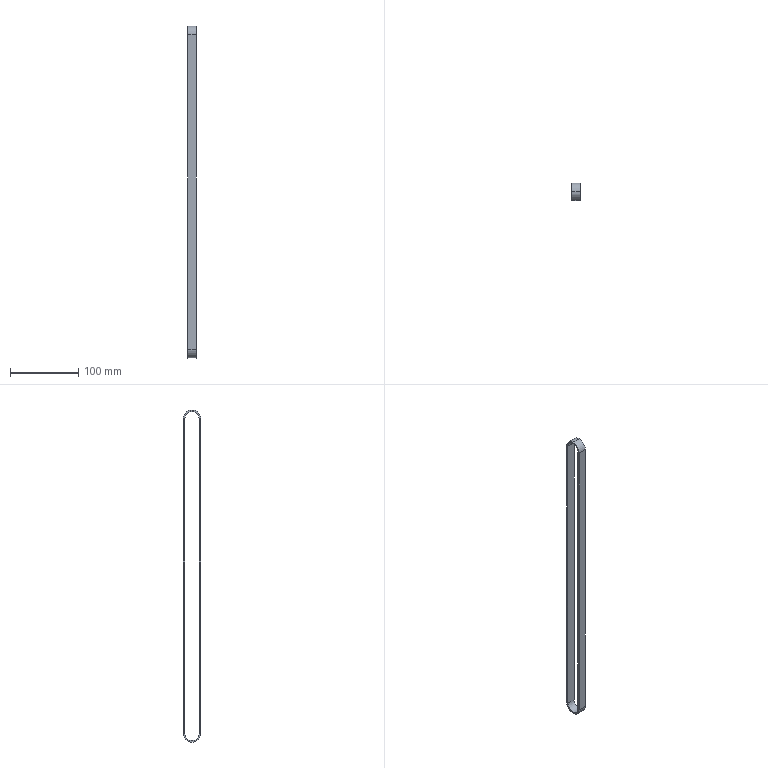Part | NX | features BREP 1 | 1 solid | 12 faces | box 12.7 x 25.408 x 484.908 mm | volume 28965 mm3 | plane 6 | cylinder 6 | commonest cylinder face diameters 20.808 x3 25.408 x3
STEP:
#1=CARTESIAN_POINT('',(-6.35,10.404,0.));
#2=VERTEX_POINT('',#1);
#3=CARTESIAN_POINT('',(6.35,10.404,0.));
#4=VERTEX_POINT('',#3);
#5=CARTESIAN_POINT('',(-6.35,10.404,0.));
#6=CARTESIAN_POINT('',(-2.117,10.404,0.));
#7=CARTESIAN_POINT('',(2.117,10.404,0.));
#8=CARTESIAN_POINT('',(6.35,10.404,0.));
#9=B_SPLINE_CURVE_WITH_KNOTS('',3,(#5,#6,#7,#8),.UNSPECIFIED.,.F.,.F.,(4,4),(0.,1.),.UNSPECIFIED.);
#10=EDGE_CURVE('',#2,#4,#9,.T.);
#11=ORIENTED_EDGE('',*,*,#10,.F.);
#12=CARTESIAN_POINT('',(-6.35,10.404,-459.5));
#13=VERTEX_POINT('',#12);
#14=CARTESIAN_POINT('',(-6.35,10.404,-459.5));
#15=DIRECTION('',(0.,0.,1.));
#16=VECTOR('',#15,1000.);
#17=LINE('',#14,#16);
#18=EDGE_CURVE('',#13,#2,#17,.T.);
#19=ORIENTED_EDGE('',*,*,#18,.F.);
#20=CARTESIAN_POINT('',(6.35,10.404,-459.5));
#21=VERTEX_POINT('',#20);
#22=CARTESIAN_POINT('',(6.35,10.404,-459.5));
#23=DIRECTION('',(1.,0.,0.));
#24=VECTOR('',#23,1000.);
#25=LINE('',#22,#24);
#26=EDGE_CURVE('',#13,#21,#25,.T.);
#27=ORIENTED_EDGE('',*,*,#26,.T.);
#28=CARTESIAN_POINT('',(6.35,10.404,-459.5));
#29=DIRECTION('',(0.,0.,1.));
#30=VECTOR('',#29,1000.);
#31=LINE('',#28,#30);
#32=EDGE_CURVE('',#21,#4,#31,.T.);
#33=ORIENTED_EDGE('',*,*,#32,.T.);
#34=EDGE_LOOP('',(#11,#19,#27,#33));
#35=FACE_BOUND('',#34,.T.);
#36=CARTESIAN_POINT('',(6.35,10.404,-459.5));
#37=DIRECTION('',(0.,-1.,0.));
#38=DIRECTION('',(0.,0.,-1.));
#39=AXIS2_PLACEMENT_3D('',#36,#37,#38);
#40=PLANE('',#39);
#41=ADVANCED_FACE('',(#35),#40,.T.);
#42=ORIENTED_EDGE('',*,*,#32,.F.);
#43=CARTESIAN_POINT('',(6.35,-10.404,-459.5));
#44=VERTEX_POINT('',#43);
#45=CARTESIAN_POINT('',(6.35,0.,-459.5));
#46=DIRECTION('',(-1.,0.,0.));
#47=DIRECTION('',(0.,0.,1.));
#48=AXIS2_PLACEMENT_3D('',#45,#46,#47);
#49=CIRCLE('',#48,10.404);
#50=EDGE_CURVE('',#21,#44,#49,.T.);
#51=ORIENTED_EDGE('',*,*,#50,.T.);
#52=CARTESIAN_POINT('',(6.35,-10.404,0.));
#53=VERTEX_POINT('',#52);
#54=CARTESIAN_POINT('',(6.35,-10.404,-459.5));
#55=DIRECTION('',(0.,0.,1.));
#56=VECTOR('',#55,1000.);
#57=LINE('',#54,#56);
#58=EDGE_CURVE('',#44,#53,#57,.T.);
#59=ORIENTED_EDGE('',*,*,#58,.T.);
#60=CARTESIAN_POINT('',(6.35,0.,10.404));
#61=VERTEX_POINT('',#60);
#62=CARTESIAN_POINT('',(6.35,0.,0.));
#63=DIRECTION('',(-1.,0.,0.));
#64=DIRECTION('',(0.,0.,1.));
#65=AXIS2_PLACEMENT_3D('',#62,#63,#64);
#66=CIRCLE('',#65,10.404);
#67=EDGE_CURVE('',#53,#61,#66,.T.);
#68=ORIENTED_EDGE('',*,*,#67,.T.);
#69=CARTESIAN_POINT('',(6.35,0.,0.));
#70=DIRECTION('',(-1.,0.,0.));
#71=DIRECTION('',(0.,0.,1.));
#72=AXIS2_PLACEMENT_3D('',#69,#70,#71);
#73=CIRCLE('',#72,10.404);
#74=EDGE_CURVE('',#61,#4,#73,.T.);
#75=ORIENTED_EDGE('',*,*,#74,.T.);
#76=EDGE_LOOP('',(#42,#51,#59,#68,#75));
#77=FACE_BOUND('',#76,.T.);
#78=CARTESIAN_POINT('',(6.35,12.704,-459.5));
#79=VERTEX_POINT('',#78);
#80=CARTESIAN_POINT('',(6.35,-12.704,-459.5));
#81=VERTEX_POINT('',#80);
#82=CARTESIAN_POINT('',(6.35,0.,-459.5));
#83=DIRECTION('',(-1.,0.,0.));
#84=DIRECTION('',(0.,0.,1.));
#85=AXIS2_PLACEMENT_3D('',#82,#83,#84);
#86=CIRCLE('',#85,12.704);
#87=EDGE_CURVE('',#79,#81,#86,.T.);
#88=ORIENTED_EDGE('',*,*,#87,.F.);
#89=CARTESIAN_POINT('',(6.35,12.704,0.));
#90=VERTEX_POINT('',#89);
#91=CARTESIAN_POINT('',(6.35,12.704,-459.5));
#92=DIRECTION('',(0.,0.,1.));
#93=VECTOR('',#92,1000.);
#94=LINE('',#91,#93);
#95=EDGE_CURVE('',#79,#90,#94,.T.);
#96=ORIENTED_EDGE('',*,*,#95,.T.);
#97=CARTESIAN_POINT('',(6.35,0.,12.704));
#98=VERTEX_POINT('',#97);
#99=CARTESIAN_POINT('',(6.35,0.,0.));
#100=DIRECTION('',(-1.,0.,0.));
#101=DIRECTION('',(0.,0.,1.));
#102=AXIS2_PLACEMENT_3D('',#99,#100,#101);
#103=CIRCLE('',#102,12.704);
#104=EDGE_CURVE('',#98,#90,#103,.T.);
#105=ORIENTED_EDGE('',*,*,#104,.F.);
#106=CARTESIAN_POINT('',(6.35,-12.704,0.));
#107=VERTEX_POINT('',#106);
#108=CARTESIAN_POINT('',(6.35,0.,0.));
#109=DIRECTION('',(-1.,0.,0.));
#110=DIRECTION('',(0.,0.,1.));
#111=AXIS2_PLACEMENT_3D('',#108,#109,#110);
#112=CIRCLE('',#111,12.704);
#113=EDGE_CURVE('',#107,#98,#112,.T.);
#114=ORIENTED_EDGE('',*,*,#113,.F.);
#115=CARTESIAN_POINT('',(6.35,-12.704,-459.5));
#116=DIRECTION('',(0.,0.,1.));
#117=VECTOR('',#116,1000.);
#118=LINE('',#115,#117);
#119=EDGE_CURVE('',#81,#107,#118,.T.);
#120=ORIENTED_EDGE('',*,*,#119,.F.);
#121=EDGE_LOOP('',(#88,#96,#105,#114,#120));
#122=FACE_BOUND('',#121,.T.);
#123=CARTESIAN_POINT('',(6.35,12.704,-459.5));
#124=DIRECTION('',(1.,0.,0.));
#125=DIRECTION('',(0.,0.,-1.));
#126=AXIS2_PLACEMENT_3D('',#123,#124,#125);
#127=PLANE('',#126);
#128=ADVANCED_FACE('',(#77,#122),#127,.T.);
#129=CARTESIAN_POINT('',(-6.35,12.704,0.));
#130=VERTEX_POINT('',#129);
#131=CARTESIAN_POINT('',(6.35,12.704,0.));
#132=CARTESIAN_POINT('',(2.117,12.704,0.));
#133=CARTESIAN_POINT('',(-2.117,12.704,0.));
#134=CARTESIAN_POINT('',(-6.35,12.704,0.));
#135=B_SPLINE_CURVE_WITH_KNOTS('',3,(#131,#132,#133,#134),.UNSPECIFIED.,.F.,.F.,(4,4),(0.,1.),.UNSPECIFIED.);
#136=EDGE_CURVE('',#90,#130,#135,.T.);
#137=ORIENTED_EDGE('',*,*,#136,.F.);
#138=ORIENTED_EDGE('',*,*,#95,.F.);
#139=CARTESIAN_POINT('',(-6.35,12.704,-459.5));
#140=VERTEX_POINT('',#139);
#141=CARTESIAN_POINT('',(-6.35,12.704,-459.5));
#142=DIRECTION('',(-1.,0.,0.));
#143=VECTOR('',#142,1000.);
#144=LINE('',#141,#143);
#145=EDGE_CURVE('',#79,#140,#144,.T.);
#146=ORIENTED_EDGE('',*,*,#145,.T.);
#147=CARTESIAN_POINT('',(-6.35,12.704,-459.5));
#148=DIRECTION('',(0.,0.,1.));
#149=VECTOR('',#148,1000.);
#150=LINE('',#147,#149);
#151=EDGE_CURVE('',#140,#130,#150,.T.);
#152=ORIENTED_EDGE('',*,*,#151,.T.);
#153=EDGE_LOOP('',(#137,#138,#146,#152));
#154=FACE_BOUND('',#153,.T.);
#155=CARTESIAN_POINT('',(-6.35,12.704,-459.5));
#156=DIRECTION('',(0.,1.,0.));
#157=DIRECTION('',(0.,0.,1.));
#158=AXIS2_PLACEMENT_3D('',#155,#156,#157);
#159=PLANE('',#158);
#160=ADVANCED_FACE('',(#154),#159,.T.);
#161=ORIENTED_EDGE('',*,*,#151,.F.);
#162=CARTESIAN_POINT('',(-6.35,-12.704,-459.5));
#163=VERTEX_POINT('',#162);
#164=CARTESIAN_POINT('',(-6.35,0.,-459.5));
#165=DIRECTION('',(-1.,0.,0.));
#166=DIRECTION('',(0.,0.,1.));
#167=AXIS2_PLACEMENT_3D('',#164,#165,#166);
#168=CIRCLE('',#167,12.704);
#169=EDGE_CURVE('',#140,#163,#168,.T.);
#170=ORIENTED_EDGE('',*,*,#169,.T.);
#171=CARTESIAN_POINT('',(-6.35,-12.704,0.));
#172=VERTEX_POINT('',#171);
#173=CARTESIAN_POINT('',(-6.35,-12.704,-459.5));
#174=DIRECTION('',(0.,0.,1.));
#175=VECTOR('',#174,1000.);
#176=LINE('',#173,#175);
#177=EDGE_CURVE('',#163,#172,#176,.T.);
#178=ORIENTED_EDGE('',*,*,#177,.T.);
#179=CARTESIAN_POINT('',(-6.35,0.,12.704));
#180=VERTEX_POINT('',#179);
#181=CARTESIAN_POINT('',(-6.35,0.,0.));
#182=DIRECTION('',(-1.,0.,0.));
#183=DIRECTION('',(0.,0.,1.));
#184=AXIS2_PLACEMENT_3D('',#181,#182,#183);
#185=CIRCLE('',#184,12.704);
#186=EDGE_CURVE('',#172,#180,#185,.T.);
#187=ORIENTED_EDGE('',*,*,#186,.T.);
#188=CARTESIAN_POINT('',(-6.35,0.,0.));
#189=DIRECTION('',(-1.,0.,0.));
#190=DIRECTION('',(0.,0.,1.));
#191=AXIS2_PLACEMENT_3D('',#188,#189,#190);
#192=CIRCLE('',#191,12.704);
#193=EDGE_CURVE('',#180,#130,#192,.T.);
#194=ORIENTED_EDGE('',*,*,#193,.T.);
#195=EDGE_LOOP('',(#161,#170,#178,#187,#194));
#196=FACE_BOUND('',#195,.T.);
#197=CARTESIAN_POINT('',(-6.35,-10.404,-459.5));
#198=VERTEX_POINT('',#197);
#199=CARTESIAN_POINT('',(-6.35,0.,-459.5));
#200=DIRECTION('',(-1.,0.,0.));
#201=DIRECTION('',(0.,0.,1.));
#202=AXIS2_PLACEMENT_3D('',#199,#200,#201);
#203=CIRCLE('',#202,10.404);
#204=EDGE_CURVE('',#13,#198,#203,.T.);
#205=ORIENTED_EDGE('',*,*,#204,.F.);
#206=ORIENTED_EDGE('',*,*,#18,.T.);
#207=CARTESIAN_POINT('',(-6.35,0.,10.404));
#208=VERTEX_POINT('',#207);
#209=CARTESIAN_POINT('',(-6.35,0.,0.));
#210=DIRECTION('',(-1.,0.,0.));
#211=DIRECTION('',(0.,0.,1.));
#212=AXIS2_PLACEMENT_3D('',#209,#210,#211);
#213=CIRCLE('',#212,10.404);
#214=EDGE_CURVE('',#208,#2,#213,.T.);
#215=ORIENTED_EDGE('',*,*,#214,.F.);
#216=CARTESIAN_POINT('',(-6.35,-10.404,0.));
#217=VERTEX_POINT('',#216);
#218=CARTESIAN_POINT('',(-6.35,0.,0.));
#219=DIRECTION('',(-1.,0.,0.));
#220=DIRECTION('',(0.,0.,1.));
#221=AXIS2_PLACEMENT_3D('',#218,#219,#220);
#222=CIRCLE('',#221,10.404);
#223=EDGE_CURVE('',#217,#208,#222,.T.);
#224=ORIENTED_EDGE('',*,*,#223,.F.);
#225=CARTESIAN_POINT('',(-6.35,-10.404,-459.5));
#226=DIRECTION('',(0.,0.,1.));
#227=VECTOR('',#226,1000.);
#228=LINE('',#225,#227);
#229=EDGE_CURVE('',#198,#217,#228,.T.);
#230=ORIENTED_EDGE('',*,*,#229,.F.);
#231=EDGE_LOOP('',(#205,#206,#215,#224,#230));
#232=FACE_BOUND('',#231,.T.);
#233=CARTESIAN_POINT('',(-6.35,10.404,-459.5));
#234=DIRECTION('',(-1.,0.,0.));
#235=DIRECTION('',(0.,0.,1.));
#236=AXIS2_PLACEMENT_3D('',#233,#234,#235);
#237=PLANE('',#236);
#238=ADVANCED_FACE('',(#196,#232),#237,.T.);
#239=ORIENTED_EDGE('',*,*,#26,.F.);
#240=ORIENTED_EDGE('',*,*,#204,.T.);
#241=CARTESIAN_POINT('',(6.35,-10.404,-459.5));
#242=DIRECTION('',(1.,0.,0.));
#243=VECTOR('',#242,1000.);
#244=LINE('',#241,#243);
#245=EDGE_CURVE('',#198,#44,#244,.T.);
#246=ORIENTED_EDGE('',*,*,#245,.T.);
#247=ORIENTED_EDGE('',*,*,#50,.F.);
#248=EDGE_LOOP('',(#239,#240,#246,#247));
#249=FACE_BOUND('',#248,.T.);
#250=CARTESIAN_POINT('',(0.,0.,-459.5));
#251=DIRECTION('',(-1.,0.,0.));
#252=DIRECTION('',(0.,0.,1.));
#253=AXIS2_PLACEMENT_3D('',#250,#251,#252);
#254=CYLINDRICAL_SURFACE('',#253,10.404);
#255=ADVANCED_FACE('',(#249),#254,.F.);
#256=ORIENTED_EDGE('',*,*,#145,.F.);
#257=ORIENTED_EDGE('',*,*,#87,.T.);
#258=CARTESIAN_POINT('',(-6.35,-12.704,-459.5));
#259=DIRECTION('',(-1.,0.,0.));
#260=VECTOR('',#259,1000.);
#261=LINE('',#258,#260);
#262=EDGE_CURVE('',#81,#163,#261,.T.);
#263=ORIENTED_EDGE('',*,*,#262,.T.);
#264=ORIENTED_EDGE('',*,*,#169,.F.);
#265=EDGE_LOOP('',(#256,#257,#263,#264));
#266=FACE_BOUND('',#265,.T.);
#267=CARTESIAN_POINT('',(0.,0.,-459.5));
#268=DIRECTION('',(-1.,0.,0.));
#269=DIRECTION('',(0.,0.,1.));
#270=AXIS2_PLACEMENT_3D('',#267,#268,#269);
#271=CYLINDRICAL_SURFACE('',#270,12.704);
#272=ADVANCED_FACE('',(#266),#271,.T.);
#273=ORIENTED_EDGE('',*,*,#245,.F.);
#274=ORIENTED_EDGE('',*,*,#229,.T.);
#275=CARTESIAN_POINT('',(6.35,-10.404,0.));
#276=DIRECTION('',(1.,0.,0.));
#277=VECTOR('',#276,1000.);
#278=LINE('',#275,#277);
#279=EDGE_CURVE('',#217,#53,#278,.T.);
#280=ORIENTED_EDGE('',*,*,#279,.T.);
#281=ORIENTED_EDGE('',*,*,#58,.F.);
#282=EDGE_LOOP('',(#273,#274,#280,#281));
#283=FACE_BOUND('',#282,.T.);
#284=CARTESIAN_POINT('',(6.35,-10.404,-459.5));
#285=DIRECTION('',(0.,-1.,0.));
#286=DIRECTION('',(0.,0.,-1.));
#287=AXIS2_PLACEMENT_3D('',#284,#285,#286);
#288=PLANE('',#287);
#289=ADVANCED_FACE('',(#283),#288,.F.);
#290=ORIENTED_EDGE('',*,*,#262,.F.);
#291=ORIENTED_EDGE('',*,*,#119,.T.);
#292=CARTESIAN_POINT('',(-6.35,-12.704,0.));
#293=DIRECTION('',(-1.,0.,0.));
#294=VECTOR('',#293,1000.);
#295=LINE('',#292,#294);
#296=EDGE_CURVE('',#107,#172,#295,.T.);
#297=ORIENTED_EDGE('',*,*,#296,.T.);
#298=ORIENTED_EDGE('',*,*,#177,.F.);
#299=EDGE_LOOP('',(#290,#291,#297,#298));
#300=FACE_BOUND('',#299,.T.);
#301=CARTESIAN_POINT('',(-6.35,-12.704,-459.5));
#302=DIRECTION('',(0.,1.,0.));
#303=DIRECTION('',(0.,0.,1.));
#304=AXIS2_PLACEMENT_3D('',#301,#302,#303);
#305=PLANE('',#304);
#306=ADVANCED_FACE('',(#300),#305,.F.);
#307=CARTESIAN_POINT('',(0.,0.,10.404));
#308=DIRECTION('',(-1.,0.,0.));
#309=VECTOR('',#308,1000.);
#310=LINE('',#307,#309);
#311=EDGE_CURVE('',#61,#208,#310,.T.);
#312=ORIENTED_EDGE('',*,*,#311,.F.);
#313=ORIENTED_EDGE('',*,*,#67,.F.);
#314=ORIENTED_EDGE('',*,*,#279,.F.);
#315=ORIENTED_EDGE('',*,*,#223,.T.);
#316=EDGE_LOOP('',(#312,#313,#314,#315));
#317=FACE_BOUND('',#316,.T.);
#318=CARTESIAN_POINT('',(0.,0.,0.));
#319=DIRECTION('',(-1.,0.,0.));
#320=DIRECTION('',(0.,0.,1.));
#321=AXIS2_PLACEMENT_3D('',#318,#319,#320);
#322=CYLINDRICAL_SURFACE('',#321,10.404);
#323=ADVANCED_FACE('',(#317),#322,.F.);
#324=CARTESIAN_POINT('',(0.,0.,12.704));
#325=DIRECTION('',(-1.,0.,0.));
#326=VECTOR('',#325,1000.);
#327=LINE('',#324,#326);
#328=EDGE_CURVE('',#98,#180,#327,.T.);
#329=ORIENTED_EDGE('',*,*,#328,.F.);
#330=ORIENTED_EDGE('',*,*,#104,.T.);
#331=ORIENTED_EDGE('',*,*,#136,.T.);
#332=ORIENTED_EDGE('',*,*,#193,.F.);
#333=EDGE_LOOP('',(#329,#330,#331,#332));
#334=FACE_BOUND('',#333,.T.);
#335=CARTESIAN_POINT('',(0.,0.,0.));
#336=DIRECTION('',(-1.,0.,0.));
#337=DIRECTION('',(0.,0.,1.));
#338=AXIS2_PLACEMENT_3D('',#335,#336,#337);
#339=CYLINDRICAL_SURFACE('',#338,12.704);
#340=ADVANCED_FACE('',(#334),#339,.T.);
#341=ORIENTED_EDGE('',*,*,#113,.T.);
#342=ORIENTED_EDGE('',*,*,#328,.T.);
#343=ORIENTED_EDGE('',*,*,#186,.F.);
#344=ORIENTED_EDGE('',*,*,#296,.F.);
#345=EDGE_LOOP('',(#341,#342,#343,#344));
#346=FACE_BOUND('',#345,.T.);
#347=CARTESIAN_POINT('',(0.,0.,0.));
#348=DIRECTION('',(-1.,0.,0.));
#349=DIRECTION('',(0.,0.,1.));
#350=AXIS2_PLACEMENT_3D('',#347,#348,#349);
#351=CYLINDRICAL_SURFACE('',#350,12.704);
#352=ADVANCED_FACE('',(#346),#351,.T.);
#353=ORIENTED_EDGE('',*,*,#74,.F.);
#354=ORIENTED_EDGE('',*,*,#311,.T.);
#355=ORIENTED_EDGE('',*,*,#214,.T.);
#356=ORIENTED_EDGE('',*,*,#10,.T.);
#357=EDGE_LOOP('',(#353,#354,#355,#356));
#358=FACE_BOUND('',#357,.T.);
#359=CARTESIAN_POINT('',(0.,0.,0.));
#360=DIRECTION('',(-1.,0.,0.));
#361=DIRECTION('',(0.,0.,1.));
#362=AXIS2_PLACEMENT_3D('',#359,#360,#361);
#363=CYLINDRICAL_SURFACE('',#362,10.404);
#364=ADVANCED_FACE('',(#358),#363,.F.);
#365=CLOSED_SHELL('',(#41,#128,#160,#238,#255,#272,#289,#306,#323,#340,#352,#364));
#366=MANIFOLD_SOLID_BREP('',#365);
#367=(LENGTH_UNIT()NAMED_UNIT(*)SI_UNIT(.MILLI.,.METRE.));
#368=UNCERTAINTY_MEASURE_WITH_UNIT(LENGTH_MEASURE(0.00001),#367,'','');
#369=(NAMED_UNIT(*)PLANE_ANGLE_UNIT()SI_UNIT($,.RADIAN.));
#370=(NAMED_UNIT(*)SI_UNIT($,.STERADIAN.)SOLID_ANGLE_UNIT());
#371=(GEOMETRIC_REPRESENTATION_CONTEXT(3)GLOBAL_UNCERTAINTY_ASSIGNED_CONTEXT((#368))GLOBAL_UNIT_ASSIGNED_CONTEXT((#367,#369,#370))REPRESENTATION_CONTEXT('',''));
#372=ADVANCED_BREP_SHAPE_REPRESENTATION('',(#366),#371);